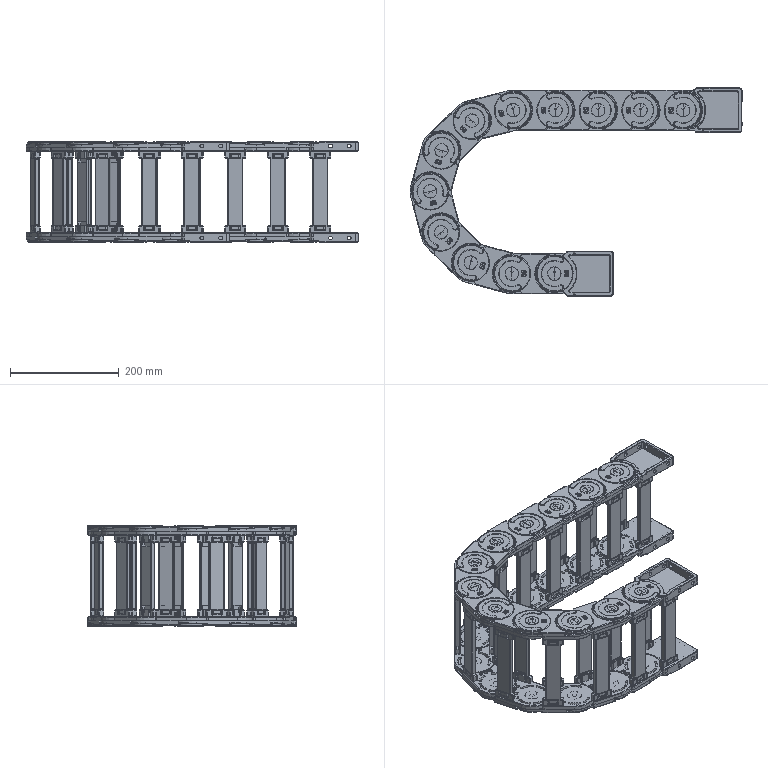Part | SolidWorks | features ReferencePattern 10, CompositeCurve 2, LocalChainPattern 1 | 52 solids | 10370 faces | volume 3103093 mm3 | plane 3744 | cylinder 2818 | cone 1232 | spline 1226 | torus 1154 | sphere 196 | commonest cylinder face diameters 3 x1040 4 x472 2 x380 6 x142 5 x96 3.2 x72